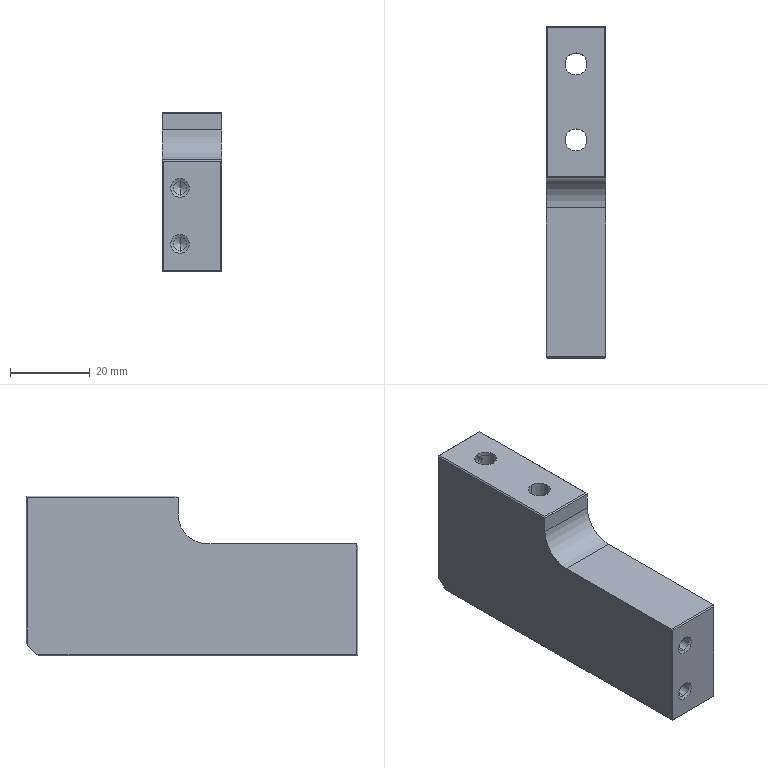Part | NX | 1 solid | 56 faces | box 15 x 83 x 39.971 mm | volume 37898 mm3 | plane 23 | cylinder 23 | cone 10 | commonest cylinder face diameters 3.3 x8 5.5 x6 2.5 x4 10 x4 15 x1